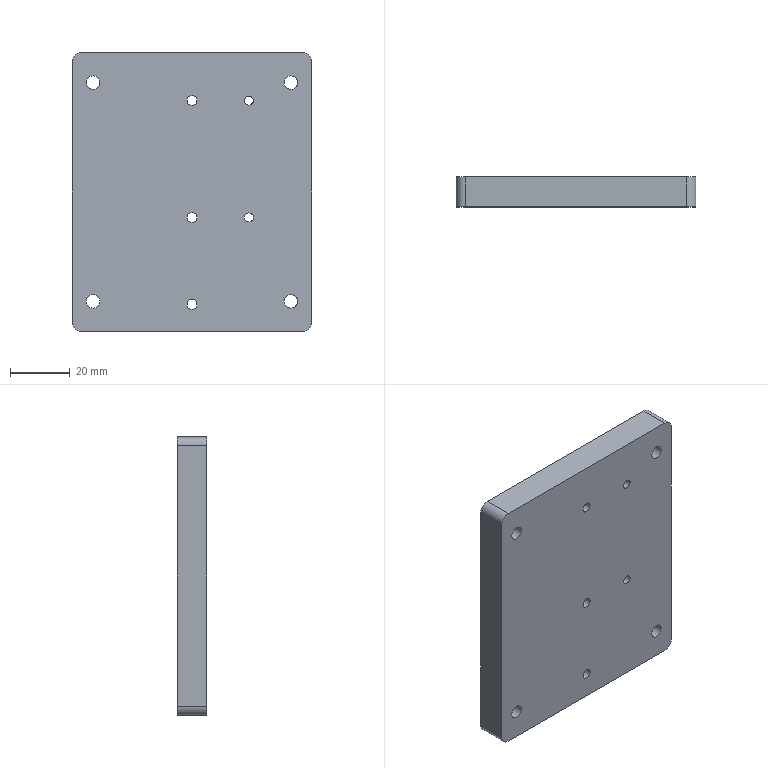Part | NX | 1 solid | 35 faces | box 80 x 10 x 93 mm | volume 72623 mm3 | cylinder 19 | plane 14 | cone 2 | commonest cylinder face diameters 4.5 x4 6 x4 8 x4 3.3 x3 3 x2 4 x2
STEP:
#1=CARTESIAN_POINT('',(104.923,-23.608,-66.529));
#2=VERTEX_POINT('',#1);
#3=CARTESIAN_POINT('',(101.923,-23.608,-69.529));
#4=VERTEX_POINT('',#3);
#5=CARTESIAN_POINT('',(104.923,-23.608,-69.529));
#6=DIRECTION('',(0.000000698,-1.,0.));
#7=DIRECTION('',(-0.000000349,0.,-1.));
#8=AXIS2_PLACEMENT_3D('',#5,#6,#7);
#9=CIRCLE('',#8,3.);
#10=EDGE_CURVE('',#2,#4,#9,.T.);
#11=ORIENTED_EDGE('',*,*,#10,.F.);
#12=CARTESIAN_POINT('',(104.923,-13.608,-66.529));
#13=VERTEX_POINT('',#12);
#14=CARTESIAN_POINT('',(104.923,-23.608,-66.529));
#15=DIRECTION('',(0.000000698,-1.,0.));
#16=VECTOR('',#15,1000.);
#17=LINE('',#14,#16);
#18=EDGE_CURVE('',#13,#2,#17,.T.);
#19=ORIENTED_EDGE('',*,*,#18,.F.);
#20=CARTESIAN_POINT('',(101.923,-13.608,-69.529));
#21=VERTEX_POINT('',#20);
#22=CARTESIAN_POINT('',(104.923,-13.608,-69.529));
#23=DIRECTION('',(-0.000000698,1.,0.));
#24=DIRECTION('',(-0.000000349,0.,-1.));
#25=AXIS2_PLACEMENT_3D('',#22,#23,#24);
#26=CIRCLE('',#25,3.);
#27=EDGE_CURVE('',#21,#13,#26,.T.);
#28=ORIENTED_EDGE('',*,*,#27,.F.);
#29=CARTESIAN_POINT('',(101.923,-24.294,-69.529));
#30=DIRECTION('',(-0.000000698,1.,0.));
#31=VECTOR('',#30,1000.);
#32=LINE('',#29,#31);
#33=EDGE_CURVE('',#4,#21,#32,.T.);
#34=ORIENTED_EDGE('',*,*,#33,.F.);
#35=EDGE_LOOP('',(#11,#19,#28,#34));
#36=FACE_BOUND('',#35,.T.);
#37=CARTESIAN_POINT('',(104.923,-23.608,-69.529));
#38=DIRECTION('',(0.000000698,-1.,0.));
#39=DIRECTION('',(-0.000000349,0.,-1.));
#40=AXIS2_PLACEMENT_3D('',#37,#38,#39);
#41=CYLINDRICAL_SURFACE('',#40,3.);
#42=ADVANCED_FACE('',(#36),#41,.T.);
#43=CARTESIAN_POINT('',(101.923,-23.608,-156.529));
#44=VERTEX_POINT('',#43);
#45=CARTESIAN_POINT('',(104.923,-23.608,-159.529));
#46=VERTEX_POINT('',#45);
#47=CARTESIAN_POINT('',(104.923,-23.608,-156.529));
#48=DIRECTION('',(0.000000698,-1.,0.));
#49=DIRECTION('',(-0.000000349,0.,-1.));
#50=AXIS2_PLACEMENT_3D('',#47,#48,#49);
#51=CIRCLE('',#50,3.);
#52=EDGE_CURVE('',#44,#46,#51,.T.);
#53=ORIENTED_EDGE('',*,*,#52,.F.);
#54=CARTESIAN_POINT('',(101.923,-13.608,-156.529));
#55=VERTEX_POINT('',#54);
#56=CARTESIAN_POINT('',(101.923,-24.294,-156.529));
#57=DIRECTION('',(0.000000698,-1.,0.));
#58=VECTOR('',#57,1000.);
#59=LINE('',#56,#58);
#60=EDGE_CURVE('',#55,#44,#59,.T.);
#61=ORIENTED_EDGE('',*,*,#60,.F.);
#62=CARTESIAN_POINT('',(104.923,-13.608,-159.529));
#63=VERTEX_POINT('',#62);
#64=CARTESIAN_POINT('',(104.923,-13.608,-156.529));
#65=DIRECTION('',(-0.000000698,1.,0.));
#66=DIRECTION('',(-0.000000349,0.,-1.));
#67=AXIS2_PLACEMENT_3D('',#64,#65,#66);
#68=CIRCLE('',#67,3.);
#69=EDGE_CURVE('',#63,#55,#68,.T.);
#70=ORIENTED_EDGE('',*,*,#69,.F.);
#71=CARTESIAN_POINT('',(104.923,-23.608,-159.529));
#72=DIRECTION('',(-0.000000698,1.,0.));
#73=VECTOR('',#72,1000.);
#74=LINE('',#71,#73);
#75=EDGE_CURVE('',#46,#63,#74,.T.);
#76=ORIENTED_EDGE('',*,*,#75,.F.);
#77=EDGE_LOOP('',(#53,#61,#70,#76));
#78=FACE_BOUND('',#77,.T.);
#79=CARTESIAN_POINT('',(104.923,-24.294,-156.529));
#80=DIRECTION('',(0.000000698,-1.,0.));
#81=DIRECTION('',(-0.000000349,0.,-1.));
#82=AXIS2_PLACEMENT_3D('',#79,#80,#81);
#83=CYLINDRICAL_SURFACE('',#82,3.);
#84=ADVANCED_FACE('',(#78),#83,.T.);
#85=CARTESIAN_POINT('',(178.923,-23.608,-159.529));
#86=VERTEX_POINT('',#85);
#87=CARTESIAN_POINT('',(181.923,-23.608,-156.529));
#88=VERTEX_POINT('',#87);
#89=CARTESIAN_POINT('',(178.923,-23.608,-156.529));
#90=DIRECTION('',(0.000000698,-1.,0.));
#91=DIRECTION('',(-0.000000349,0.,-1.));
#92=AXIS2_PLACEMENT_3D('',#89,#90,#91);
#93=CIRCLE('',#92,3.);
#94=EDGE_CURVE('',#86,#88,#93,.T.);
#95=ORIENTED_EDGE('',*,*,#94,.F.);
#96=CARTESIAN_POINT('',(178.923,-13.608,-159.529));
#97=VERTEX_POINT('',#96);
#98=CARTESIAN_POINT('',(178.923,-23.608,-159.529));
#99=DIRECTION('',(0.000000698,-1.,0.));
#100=VECTOR('',#99,1000.);
#101=LINE('',#98,#100);
#102=EDGE_CURVE('',#97,#86,#101,.T.);
#103=ORIENTED_EDGE('',*,*,#102,.F.);
#104=CARTESIAN_POINT('',(181.923,-13.608,-156.529));
#105=VERTEX_POINT('',#104);
#106=CARTESIAN_POINT('',(178.923,-13.608,-156.529));
#107=DIRECTION('',(-0.000000698,1.,0.));
#108=DIRECTION('',(-0.000000349,0.,-1.));
#109=AXIS2_PLACEMENT_3D('',#106,#107,#108);
#110=CIRCLE('',#109,3.);
#111=EDGE_CURVE('',#105,#97,#110,.T.);
#112=ORIENTED_EDGE('',*,*,#111,.F.);
#113=CARTESIAN_POINT('',(181.923,-24.294,-156.529));
#114=DIRECTION('',(-0.000000698,1.,0.));
#115=VECTOR('',#114,1000.);
#116=LINE('',#113,#115);
#117=EDGE_CURVE('',#88,#105,#116,.T.);
#118=ORIENTED_EDGE('',*,*,#117,.F.);
#119=EDGE_LOOP('',(#95,#103,#112,#118));
#120=FACE_BOUND('',#119,.T.);
#121=CARTESIAN_POINT('',(178.923,-23.608,-156.529));
#122=DIRECTION('',(-0.000000698,1.,0.));
#123=DIRECTION('',(0.000000349,0.,1.));
#124=AXIS2_PLACEMENT_3D('',#121,#122,#123);
#125=CYLINDRICAL_SURFACE('',#124,3.);
#126=ADVANCED_FACE('',(#120),#125,.T.);
#127=CARTESIAN_POINT('',(181.923,-23.608,-69.529));
#128=VERTEX_POINT('',#127);
#129=CARTESIAN_POINT('',(178.923,-23.608,-66.529));
#130=VERTEX_POINT('',#129);
#131=CARTESIAN_POINT('',(178.923,-23.608,-69.529));
#132=DIRECTION('',(0.000000698,-1.,0.));
#133=DIRECTION('',(-0.000000349,0.,-1.));
#134=AXIS2_PLACEMENT_3D('',#131,#132,#133);
#135=CIRCLE('',#134,3.);
#136=EDGE_CURVE('',#128,#130,#135,.T.);
#137=ORIENTED_EDGE('',*,*,#136,.F.);
#138=CARTESIAN_POINT('',(181.923,-13.608,-69.529));
#139=VERTEX_POINT('',#138);
#140=CARTESIAN_POINT('',(181.923,-24.294,-69.529));
#141=DIRECTION('',(0.000000698,-1.,0.));
#142=VECTOR('',#141,1000.);
#143=LINE('',#140,#142);
#144=EDGE_CURVE('',#139,#128,#143,.T.);
#145=ORIENTED_EDGE('',*,*,#144,.F.);
#146=CARTESIAN_POINT('',(178.923,-13.608,-66.529));
#147=VERTEX_POINT('',#146);
#148=CARTESIAN_POINT('',(178.923,-13.608,-69.529));
#149=DIRECTION('',(-0.000000698,1.,0.));
#150=DIRECTION('',(-0.000000349,0.,-1.));
#151=AXIS2_PLACEMENT_3D('',#148,#149,#150);
#152=CIRCLE('',#151,3.);
#153=EDGE_CURVE('',#147,#139,#152,.T.);
#154=ORIENTED_EDGE('',*,*,#153,.F.);
#155=CARTESIAN_POINT('',(178.923,-23.608,-66.529));
#156=DIRECTION('',(-0.000000698,1.,0.));
#157=VECTOR('',#156,1000.);
#158=LINE('',#155,#157);
#159=EDGE_CURVE('',#130,#147,#158,.T.);
#160=ORIENTED_EDGE('',*,*,#159,.F.);
#161=EDGE_LOOP('',(#137,#145,#154,#160));
#162=FACE_BOUND('',#161,.T.);
#163=CARTESIAN_POINT('',(178.923,-24.294,-69.529));
#164=DIRECTION('',(-0.000000698,1.,0.));
#165=DIRECTION('',(0.000000349,0.,1.));
#166=AXIS2_PLACEMENT_3D('',#163,#164,#165);
#167=CYLINDRICAL_SURFACE('',#166,3.);
#168=ADVANCED_FACE('',(#162),#167,.T.);
#169=CARTESIAN_POINT('',(162.923,-18.608,-82.529));
#170=VERTEX_POINT('',#169);
#171=CARTESIAN_POINT('',(160.923,-18.608,-82.529));
#172=DIRECTION('',(-0.000000698,1.,0.));
#173=DIRECTION('',(1.,0.000000698,0.));
#174=AXIS2_PLACEMENT_3D('',#171,#172,#173);
#175=CIRCLE('',#174,2.);
#176=EDGE_CURVE('',#170,#170,#175,.T.);
#177=ORIENTED_EDGE('',*,*,#176,.T.);
#178=EDGE_LOOP('',(#177));
#179=FACE_BOUND('',#178,.T.);
#180=CARTESIAN_POINT('',(162.423,-18.608,-82.529));
#181=VERTEX_POINT('',#180);
#182=CARTESIAN_POINT('',(160.923,-18.608,-82.529));
#183=DIRECTION('',(-0.000000698,1.,0.));
#184=DIRECTION('',(1.,0.000000698,0.));
#185=AXIS2_PLACEMENT_3D('',#182,#183,#184);
#186=CIRCLE('',#185,1.5);
#187=EDGE_CURVE('',#181,#181,#186,.T.);
#188=ORIENTED_EDGE('',*,*,#187,.F.);
#189=EDGE_LOOP('',(#188));
#190=FACE_BOUND('',#189,.T.);
#191=CARTESIAN_POINT('',(160.923,-18.608,-123.029));
#192=DIRECTION('',(0.000000698,-1.,0.));
#193=DIRECTION('',(0.,0.,-1.));
#194=AXIS2_PLACEMENT_3D('',#191,#192,#193);
#195=PLANE('',#194);
#196=ADVANCED_FACE('',(#179,#190),#195,.F.);
#197=CARTESIAN_POINT('',(160.923,-18.608,-119.529));
#198=VERTEX_POINT('',#197);
#199=CARTESIAN_POINT('',(160.923,-18.608,-121.529));
#200=DIRECTION('',(-0.000000698,1.,0.));
#201=DIRECTION('',(0.,0.,1.));
#202=AXIS2_PLACEMENT_3D('',#199,#200,#201);
#203=CIRCLE('',#202,2.);
#204=EDGE_CURVE('',#198,#198,#203,.T.);
#205=ORIENTED_EDGE('',*,*,#204,.T.);
#206=EDGE_LOOP('',(#205));
#207=FACE_BOUND('',#206,.T.);
#208=CARTESIAN_POINT('',(160.923,-18.608,-120.029));
#209=VERTEX_POINT('',#208);
#210=CARTESIAN_POINT('',(160.923,-18.608,-121.529));
#211=DIRECTION('',(-0.000000698,1.,0.));
#212=DIRECTION('',(0.,0.,1.));
#213=AXIS2_PLACEMENT_3D('',#210,#211,#212);
#214=CIRCLE('',#213,1.5);
#215=EDGE_CURVE('',#209,#209,#214,.T.);
#216=ORIENTED_EDGE('',*,*,#215,.F.);
#217=EDGE_LOOP('',(#216));
#218=FACE_BOUND('',#217,.T.);
#219=CARTESIAN_POINT('',(160.923,-18.608,-123.029));
#220=DIRECTION('',(0.000000698,-1.,0.));
#221=DIRECTION('',(0.,0.,-1.));
#222=AXIS2_PLACEMENT_3D('',#219,#220,#221);
#223=PLANE('',#222);
#224=ADVANCED_FACE('',(#207,#218),#223,.F.);
#225=CARTESIAN_POINT('',(178.923,-18.008,-149.529));
#226=VERTEX_POINT('',#225);
#227=CARTESIAN_POINT('',(174.923,-18.008,-149.529));
#228=DIRECTION('',(-0.000000698,1.,0.));
#229=DIRECTION('',(1.,0.000000698,0.));
#230=AXIS2_PLACEMENT_3D('',#227,#228,#229);
#231=CIRCLE('',#230,4.);
#232=EDGE_CURVE('',#226,#226,#231,.T.);
#233=ORIENTED_EDGE('',*,*,#232,.T.);
#234=EDGE_LOOP('',(#233));
#235=FACE_BOUND('',#234,.T.);
#236=CARTESIAN_POINT('',(177.173,-18.008,-149.529));
#237=VERTEX_POINT('',#236);
#238=CARTESIAN_POINT('',(174.923,-18.008,-149.529));
#239=DIRECTION('',(-0.000000698,1.,0.));
#240=DIRECTION('',(1.,0.000000698,0.));
#241=AXIS2_PLACEMENT_3D('',#238,#239,#240);
#242=CIRCLE('',#241,2.25);
#243=EDGE_CURVE('',#237,#237,#242,.T.);
#244=ORIENTED_EDGE('',*,*,#243,.F.);
#245=EDGE_LOOP('',(#244));
#246=FACE_BOUND('',#245,.T.);
#247=CARTESIAN_POINT('',(108.923,-18.008,-151.779));
#248=DIRECTION('',(0.000000698,-1.,0.));
#249=DIRECTION('',(0.,0.,-1.));
#250=AXIS2_PLACEMENT_3D('',#247,#248,#249);
#251=PLANE('',#250);
#252=ADVANCED_FACE('',(#235,#246),#251,.F.);
#253=CARTESIAN_POINT('',(178.923,-18.008,-76.529));
#254=VERTEX_POINT('',#253);
#255=CARTESIAN_POINT('',(174.923,-18.008,-76.529));
#256=DIRECTION('',(-0.000000698,1.,0.));
#257=DIRECTION('',(1.,0.000000698,0.));
#258=AXIS2_PLACEMENT_3D('',#255,#256,#257);
#259=CIRCLE('',#258,4.);
#260=EDGE_CURVE('',#254,#254,#259,.T.);
#261=ORIENTED_EDGE('',*,*,#260,.T.);
#262=EDGE_LOOP('',(#261));
#263=FACE_BOUND('',#262,.T.);
#264=CARTESIAN_POINT('',(177.173,-18.008,-76.529));
#265=VERTEX_POINT('',#264);
#266=CARTESIAN_POINT('',(174.923,-18.008,-76.529));
#267=DIRECTION('',(-0.000000698,1.,0.));
#268=DIRECTION('',(1.,0.000000698,0.));
#269=AXIS2_PLACEMENT_3D('',#266,#267,#268);
#270=CIRCLE('',#269,2.25);
#271=EDGE_CURVE('',#265,#265,#270,.T.);
#272=ORIENTED_EDGE('',*,*,#271,.F.);
#273=EDGE_LOOP('',(#272));
#274=FACE_BOUND('',#273,.T.);
#275=CARTESIAN_POINT('',(108.923,-18.008,-151.779));
#276=DIRECTION('',(0.000000698,-1.,0.));
#277=DIRECTION('',(0.,0.,-1.));
#278=AXIS2_PLACEMENT_3D('',#275,#276,#277);
#279=PLANE('',#278);
#280=ADVANCED_FACE('',(#263,#274),#279,.F.);
#281=CARTESIAN_POINT('',(112.923,-18.008,-76.529));
#282=VERTEX_POINT('',#281);
#283=CARTESIAN_POINT('',(108.923,-18.008,-76.529));
#284=DIRECTION('',(-0.000000698,1.,0.));
#285=DIRECTION('',(1.,0.000000698,0.));
#286=AXIS2_PLACEMENT_3D('',#283,#284,#285);
#287=CIRCLE('',#286,4.);
#288=EDGE_CURVE('',#282,#282,#287,.T.);
#289=ORIENTED_EDGE('',*,*,#288,.T.);
#290=EDGE_LOOP('',(#289));
#291=FACE_BOUND('',#290,.T.);
#292=CARTESIAN_POINT('',(111.173,-18.008,-76.529));
#293=VERTEX_POINT('',#292);
#294=CARTESIAN_POINT('',(108.923,-18.008,-76.529));
#295=DIRECTION('',(-0.000000698,1.,0.));
#296=DIRECTION('',(1.,0.000000698,0.));
#297=AXIS2_PLACEMENT_3D('',#294,#295,#296);
#298=CIRCLE('',#297,2.25);
#299=EDGE_CURVE('',#293,#293,#298,.T.);
#300=ORIENTED_EDGE('',*,*,#299,.F.);
#301=EDGE_LOOP('',(#300));
#302=FACE_BOUND('',#301,.T.);
#303=CARTESIAN_POINT('',(108.923,-18.008,-151.779));
#304=DIRECTION('',(0.000000698,-1.,0.));
#305=DIRECTION('',(0.,0.,-1.));
#306=AXIS2_PLACEMENT_3D('',#303,#304,#305);
#307=PLANE('',#306);
#308=ADVANCED_FACE('',(#291,#302),#307,.F.);
#309=CARTESIAN_POINT('',(108.923,-18.008,-145.529));
#310=VERTEX_POINT('',#309);
#311=CARTESIAN_POINT('',(108.923,-18.008,-149.529));
#312=DIRECTION('',(-0.000000698,1.,0.));
#313=DIRECTION('',(0.,0.,1.));
#314=AXIS2_PLACEMENT_3D('',#311,#312,#313);
#315=CIRCLE('',#314,4.);
#316=EDGE_CURVE('',#310,#310,#315,.T.);
#317=ORIENTED_EDGE('',*,*,#316,.T.);
#318=EDGE_LOOP('',(#317));
#319=FACE_BOUND('',#318,.T.);
#320=CARTESIAN_POINT('',(108.923,-18.008,-147.279));
#321=VERTEX_POINT('',#320);
#322=CARTESIAN_POINT('',(108.923,-18.008,-149.529));
#323=DIRECTION('',(-0.000000698,1.,0.));
#324=DIRECTION('',(0.,0.,1.));
#325=AXIS2_PLACEMENT_3D('',#322,#323,#324);
#326=CIRCLE('',#325,2.25);
#327=EDGE_CURVE('',#321,#321,#326,.T.);
#328=ORIENTED_EDGE('',*,*,#327,.F.);
#329=EDGE_LOOP('',(#328));
#330=FACE_BOUND('',#329,.T.);
#331=CARTESIAN_POINT('',(108.923,-18.008,-151.779));
#332=DIRECTION('',(0.000000698,-1.,0.));
#333=DIRECTION('',(0.,0.,-1.));
#334=AXIS2_PLACEMENT_3D('',#331,#332,#333);
#335=PLANE('',#334);
#336=ADVANCED_FACE('',(#319,#330),#335,.F.);
#337=CARTESIAN_POINT('',(105.923,-13.608,-66.529));
#338=DIRECTION('',(-1.,-0.000000698,0.));
#339=VECTOR('',#338,1000.);
#340=LINE('',#337,#339);
#341=EDGE_CURVE('',#147,#13,#340,.T.);
#342=ORIENTED_EDGE('',*,*,#341,.F.);
#343=ORIENTED_EDGE('',*,*,#153,.T.);
#344=CARTESIAN_POINT('',(181.923,-13.608,-112.251));
#345=DIRECTION('',(0.,0.,1.));
#346=VECTOR('',#345,1000.);
#347=LINE('',#344,#346);
#348=EDGE_CURVE('',#105,#139,#347,.T.);
#349=ORIENTED_EDGE('',*,*,#348,.F.);
#350=ORIENTED_EDGE('',*,*,#111,.T.);
#351=CARTESIAN_POINT('',(105.923,-13.608,-159.529));
#352=DIRECTION('',(1.,0.000000698,0.));
#353=VECTOR('',#352,1000.);
#354=LINE('',#351,#353);
#355=EDGE_CURVE('',#63,#97,#354,.T.);
#356=ORIENTED_EDGE('',*,*,#355,.F.);
#357=ORIENTED_EDGE('',*,*,#69,.T.);
#358=CARTESIAN_POINT('',(101.923,-13.608,-112.251));
#359=DIRECTION('',(0.,0.,-1.));
#360=VECTOR('',#359,1000.);
#361=LINE('',#358,#360);
#362=EDGE_CURVE('',#21,#55,#361,.T.);
#363=ORIENTED_EDGE('',*,*,#362,.F.);
#364=ORIENTED_EDGE('',*,*,#27,.T.);
#365=EDGE_LOOP('',(#342,#343,#349,#350,#356,#357,#363,#364));
#366=FACE_BOUND('',#365,.T.);
#367=CARTESIAN_POINT('',(141.923,-13.608,-80.879));
#368=VERTEX_POINT('',#367);
#369=CARTESIAN_POINT('',(141.923,-13.608,-82.529));
#370=DIRECTION('',(-0.000000698,1.,0.));
#371=DIRECTION('',(0.,0.,1.));
#372=AXIS2_PLACEMENT_3D('',#369,#370,#371);
#373=CIRCLE('',#372,1.65);
#374=EDGE_CURVE('',#368,#368,#373,.T.);
#375=ORIENTED_EDGE('',*,*,#374,.F.);
#376=EDGE_LOOP('',(#375));
#377=FACE_BOUND('',#376,.T.);
#378=CARTESIAN_POINT('',(141.923,-13.608,-148.879));
#379=VERTEX_POINT('',#378);
#380=CARTESIAN_POINT('',(141.923,-13.608,-150.529));
#381=DIRECTION('',(-0.000000698,1.,0.));
#382=DIRECTION('',(0.,0.,1.));
#383=AXIS2_PLACEMENT_3D('',#380,#381,#382);
#384=CIRCLE('',#383,1.65);
#385=EDGE_CURVE('',#379,#379,#384,.T.);
#386=ORIENTED_EDGE('',*,*,#385,.F.);
#387=EDGE_LOOP('',(#386));
#388=FACE_BOUND('',#387,.T.);
#389=CARTESIAN_POINT('',(141.923,-13.608,-119.879));
#390=VERTEX_POINT('',#389);
#391=CARTESIAN_POINT('',(141.923,-13.608,-121.529));
#392=DIRECTION('',(-0.000000698,1.,0.));
#393=DIRECTION('',(0.,0.,1.));
#394=AXIS2_PLACEMENT_3D('',#391,#392,#393);
#395=CIRCLE('',#394,1.65);
#396=EDGE_CURVE('',#390,#390,#395,.T.);
#397=ORIENTED_EDGE('',*,*,#396,.F.);
#398=EDGE_LOOP('',(#397));
#399=FACE_BOUND('',#398,.T.);
#400=CARTESIAN_POINT('',(108.923,-13.608,-145.529));
#401=VERTEX_POINT('',#400);
#402=CARTESIAN_POINT('',(108.923,-13.608,-149.529));
#403=DIRECTION('',(-0.000000698,1.,0.));
#404=DIRECTION('',(0.,0.,1.));
#405=AXIS2_PLACEMENT_3D('',#402,#403,#404);
#406=CIRCLE('',#405,4.);
#407=EDGE_CURVE('',#401,#401,#406,.T.);
#408=ORIENTED_EDGE('',*,*,#407,.F.);
#409=EDGE_LOOP('',(#408));
#410=FACE_BOUND('',#409,.T.);
#411=CARTESIAN_POINT('',(108.923,-13.608,-72.529));
#412=VERTEX_POINT('',#411);
#413=CARTESIAN_POINT('',(108.923,-13.608,-76.529));
#414=DIRECTION('',(-0.000000698,1.,0.));
#415=DIRECTION('',(0.,0.,1.));
#416=AXIS2_PLACEMENT_3D('',#413,#414,#415);
#417=CIRCLE('',#416,4.);
#418=EDGE_CURVE('',#412,#412,#417,.T.);
#419=ORIENTED_EDGE('',*,*,#418,.F.);
#420=EDGE_LOOP('',(#419));
#421=FACE_BOUND('',#420,.T.);
#422=CARTESIAN_POINT('',(174.923,-13.608,-72.529));
#423=VERTEX_POINT('',#422);
#424=CARTESIAN_POINT('',(174.923,-13.608,-76.529));
#425=DIRECTION('',(-0.000000698,1.,0.));
#426=DIRECTION('',(0.,0.,1.));
#427=AXIS2_PLACEMENT_3D('',#424,#425,#426);
#428=CIRCLE('',#427,4.);
#429=EDGE_CURVE('',#423,#423,#428,.T.);
#430=ORIENTED_EDGE('',*,*,#429,.F.);
#431=EDGE_LOOP('',(#430));
#432=FACE_BOUND('',#431,.T.);
#433=CARTESIAN_POINT('',(174.923,-13.608,-145.529));
#434=VERTEX_POINT('',#433);
#435=CARTESIAN_POINT('',(174.923,-13.608,-149.529));
#436=DIRECTION('',(-0.000000698,1.,0.));
#437=DIRECTION('',(0.,0.,1.));
#438=AXIS2_PLACEMENT_3D('',#435,#436,#437);
#439=CIRCLE('',#438,4.);
#440=EDGE_CURVE('',#434,#434,#439,.T.);
#441=ORIENTED_EDGE('',*,*,#440,.F.);
#442=EDGE_LOOP('',(#441));
#443=FACE_BOUND('',#442,.T.);
#444=CARTESIAN_POINT('',(160.923,-13.608,-119.529));
#445=VERTEX_POINT('',#444);
#446=CARTESIAN_POINT('',(160.923,-13.608,-121.529));
#447=DIRECTION('',(-0.000000698,1.,0.));
#448=DIRECTION('',(0.,0.,1.));
#449=AXIS2_PLACEMENT_3D('',#446,#447,#448);
#450=CIRCLE('',#449,2.);
#451=EDGE_CURVE('',#445,#445,#450,.T.);
#452=ORIENTED_EDGE('',*,*,#451,.F.);
#453=EDGE_LOOP('',(#452));
#454=FACE_BOUND('',#453,.T.);
#455=CARTESIAN_POINT('',(160.923,-13.608,-80.529));
#456=VERTEX_POINT('',#455);
#457=CARTESIAN_POINT('',(160.923,-13.608,-82.529));
#458=DIRECTION('',(-0.000000698,1.,0.));
#459=DIRECTION('',(0.,0.,1.));
#460=AXIS2_PLACEMENT_3D('',#457,#458,#459);
#461=CIRCLE('',#460,2.);
#462=EDGE_CURVE('',#456,#456,#461,.T.);
#463=ORIENTED_EDGE('',*,*,#462,.F.);
#464=EDGE_LOOP('',(#463));
#465=FACE_BOUND('',#464,.T.);
#466=CARTESIAN_POINT('',(141.923,-13.608,-113.029));
#467=DIRECTION('',(0.000000698,-1.,0.));
#468=DIRECTION('',(0.,0.,-1.));
#469=AXIS2_PLACEMENT_3D('',#466,#467,#468);
#470=PLANE('',#469);
#471=ADVANCED_FACE('',(#366,#377,#388,#399,#410,#421,#432,#443,#454,#465),#470,.F.);
#472=CARTESIAN_POINT('',(181.923,-23.608,-112.251));
#473=DIRECTION('',(0.,0.,1.));
#474=VECTOR('',#473,1000.);
#475=LINE('',#472,#474);
#476=EDGE_CURVE('',#88,#128,#475,.T.);
#477=ORIENTED_EDGE('',*,*,#476,.T.);
#478=ORIENTED_EDGE('',*,*,#136,.T.);
#479=CARTESIAN_POINT('',(105.923,-23.608,-66.529));
#480=DIRECTION('',(-1.,-0.000000698,0.));
#481=VECTOR('',#480,1000.);
#482=LINE('',#479,#481);
#483=EDGE_CURVE('',#130,#2,#482,.T.);
#484=ORIENTED_EDGE('',*,*,#483,.T.);
#485=ORIENTED_EDGE('',*,*,#10,.T.);
#486=CARTESIAN_POINT('',(101.923,-23.608,-112.251));
#487=DIRECTION('',(0.,0.,-1.));
#488=VECTOR('',#487,1000.);
#489=LINE('',#486,#488);
#490=EDGE_CURVE('',#4,#44,#489,.T.);
#491=ORIENTED_EDGE('',*,*,#490,.T.);
#492=ORIENTED_EDGE('',*,*,#52,.T.);
#493=CARTESIAN_POINT('',(105.923,-23.608,-159.529));
#494=DIRECTION('',(1.,0.000000698,0.));
#495=VECTOR('',#494,1000.);
#496=LINE('',#493,#495);
#497=EDGE_CURVE('',#46,#86,#496,.T.);
#498=ORIENTED_EDGE('',*,*,#497,.T.);
#499=ORIENTED_EDGE('',*,*,#94,.T.);
#500=EDGE_LOOP('',(#477,#478,#484,#485,#491,#492,#498,#499));
#501=FACE_BOUND('',#500,.T.);
#502=CARTESIAN_POINT('',(141.923,-23.608,-80.879));
#503=VERTEX_POINT('',#502);
#504=CARTESIAN_POINT('',(141.923,-23.608,-82.529));
#505=DIRECTION('',(-0.000000698,1.,0.));
#506=DIRECTION('',(0.,0.,1.));
#507=AXIS2_PLACEMENT_3D('',#504,#505,#506);
#508=CIRCLE('',#507,1.65);
#509=EDGE_CURVE('',#503,#503,#508,.T.);
#510=ORIENTED_EDGE('',*,*,#509,.T.);
#511=EDGE_LOOP('',(#510));
#512=FACE_BOUND('',#511,.T.);
#513=CARTESIAN_POINT('',(141.923,-23.608,-148.879));
#514=VERTEX_POINT('',#513);
#515=CARTESIAN_POINT('',(141.923,-23.608,-150.529));
#516=DIRECTION('',(-0.000000698,1.,0.));
#517=DIRECTION('',(0.,0.,1.));
#518=AXIS2_PLACEMENT_3D('',#515,#516,#517);
#519=CIRCLE('',#518,1.65);
#520=EDGE_CURVE('',#514,#514,#519,.T.);
#521=ORIENTED_EDGE('',*,*,#520,.T.);
#522=EDGE_LOOP('',(#521));
#523=FACE_BOUND('',#522,.T.);
#524=CARTESIAN_POINT('',(141.923,-23.608,-119.879));
#525=VERTEX_POINT('',#524);
#526=CARTESIAN_POINT('',(141.923,-23.608,-121.529));
#527=DIRECTION('',(-0.000000698,1.,0.));
#528=DIRECTION('',(0.,0.,1.));
#529=AXIS2_PLACEMENT_3D('',#526,#527,#528);
#530=CIRCLE('',#529,1.65);
#531=EDGE_CURVE('',#525,#525,#530,.T.);
#532=ORIENTED_EDGE('',*,*,#531,.T.);
#533=EDGE_LOOP('',(#532));
#534=FACE_BOUND('',#533,.T.);
#535=CARTESIAN_POINT('',(108.923,-23.608,-147.279));
#536=VERTEX_POINT('',#535);
#537=CARTESIAN_POINT('',(108.923,-23.608,-149.529));
#538=DIRECTION('',(-0.000000698,1.,0.));
#539=DIRECTION('',(0.,0.,1.));
#540=AXIS2_PLACEMENT_3D('',#537,#538,#539);
#541=CIRCLE('',#540,2.25);
#542=EDGE_CURVE('',#536,#536,#541,.T.);
#543=ORIENTED_EDGE('',*,*,#542,.T.);
#544=EDGE_LOOP('',(#543));
#545=FACE_BOUND('',#544,.T.);
#546=CARTESIAN_POINT('',(108.923,-23.608,-74.279));
#547=VERTEX_POINT('',#546);
#548=CARTESIAN_POINT('',(108.923,-23.608,-76.529));
#549=DIRECTION('',(-0.000000698,1.,0.));
#550=DIRECTION('',(0.,0.,1.));
#551=AXIS2_PLACEMENT_3D('',#548,#549,#550);
#552=CIRCLE('',#551,2.25);
#553=EDGE_CURVE('',#547,#547,#552,.T.);
#554=ORIENTED_EDGE('',*,*,#553,.T.);
#555=EDGE_LOOP('',(#554));
#556=FACE_BOUND('',#555,.T.);
#557=CARTESIAN_POINT('',(174.923,-23.608,-74.279));
#558=VERTEX_POINT('',#557);
#559=CARTESIAN_POINT('',(174.923,-23.608,-76.529));
#560=DIRECTION('',(-0.000000698,1.,0.));
#561=DIRECTION('',(0.,0.,1.));
#562=AXIS2_PLACEMENT_3D('',#559,#560,#561);
#563=CIRCLE('',#562,2.25);
#564=EDGE_CURVE('',#558,#558,#563,.T.);
#565=ORIENTED_EDGE('',*,*,#564,.T.);
#566=EDGE_LOOP('',(#565));
#567=FACE_BOUND('',#566,.T.);
#568=CARTESIAN_POINT('',(174.923,-23.608,-147.279));
#569=VERTEX_POINT('',#568);
#570=CARTESIAN_POINT('',(174.923,-23.608,-149.529));
#571=DIRECTION('',(-0.000000698,1.,0.));
#572=DIRECTION('',(0.,0.,1.));
#573=AXIS2_PLACEMENT_3D('',#570,#571,#572);
#574=CIRCLE('',#573,2.25);
#575=EDGE_CURVE('',#569,#569,#574,.T.);
#576=ORIENTED_EDGE('',*,*,#575,.T.);
#577=EDGE_LOOP('',(#576));
#578=FACE_BOUND('',#577,.T.);
#579=CARTESIAN_POINT('',(160.923,-23.608,-120.029));
#580=VERTEX_POINT('',#579);
#581=CARTESIAN_POINT('',(160.923,-23.608,-121.529));
#582=DIRECTION('',(-0.000000698,1.,0.));
#583=DIRECTION('',(0.,0.,1.));
#584=AXIS2_PLACEMENT_3D('',#581,#582,#583);
#585=CIRCLE('',#584,1.5);
#586=EDGE_CURVE('',#580,#580,#585,.T.);
#587=ORIENTED_EDGE('',*,*,#586,.T.);
#588=EDGE_LOOP('',(#587));
#589=FACE_BOUND('',#588,.T.);
#590=CARTESIAN_POINT('',(160.923,-23.608,-81.029));
#591=VERTEX_POINT('',#590);
#592=CARTESIAN_POINT('',(160.923,-23.608,-82.529));
#593=DIRECTION('',(-0.000000698,1.,0.));
#594=DIRECTION('',(0.,0.,1.));
#595=AXIS2_PLACEMENT_3D('',#592,#593,#594);
#596=CIRCLE('',#595,1.5);
#597=EDGE_CURVE('',#591,#591,#596,.T.);
#598=ORIENTED_EDGE('',*,*,#597,.T.);
#599=EDGE_LOOP('',(#598));
#600=FACE_BOUND('',#599,.T.);
#601=CARTESIAN_POINT('',(141.923,-23.608,-113.029));
#602=DIRECTION('',(0.000000698,-1.,0.));
#603=DIRECTION('',(0.,0.,-1.));
#604=AXIS2_PLACEMENT_3D('',#601,#602,#603);
#605=PLANE('',#604);
#606=ADVANCED_FACE('',(#501,#512,#523,#534,#545,#556,#567,#578,#589,#600),#605,.T.);
#607=ORIENTED_EDGE('',*,*,#348,.T.);
#608=ORIENTED_EDGE('',*,*,#144,.T.);
#609=ORIENTED_EDGE('',*,*,#476,.F.);
#610=ORIENTED_EDGE('',*,*,#117,.T.);
#611=EDGE_LOOP('',(#607,#608,#609,#610));
#612=FACE_BOUND('',#611,.T.);
#613=CARTESIAN_POINT('',(181.923,-24.294,-112.251));
#614=DIRECTION('',(1.,0.000000698,0.));
#615=DIRECTION('',(0.,0.,-1.));
#616=AXIS2_PLACEMENT_3D('',#613,#614,#615);
#617=PLANE('',#616);
#618=ADVANCED_FACE('',(#612),#617,.T.);
#619=ORIENTED_EDGE('',*,*,#355,.T.);
#620=ORIENTED_EDGE('',*,*,#102,.T.);
#621=ORIENTED_EDGE('',*,*,#497,.F.);
#622=ORIENTED_EDGE('',*,*,#75,.T.);
#623=EDGE_LOOP('',(#619,#620,#621,#622));
#624=FACE_BOUND('',#623,.T.);
#625=CARTESIAN_POINT('',(105.923,-23.608,-159.529));
#626=DIRECTION('',(0.,0.,1.));
#627=DIRECTION('',(1.,0.,0.));
#628=AXIS2_PLACEMENT_3D('',#625,#626,#627);
#629=PLANE('',#628);
#630=ADVANCED_FACE('',(#624),#629,.F.);
#631=ORIENTED_EDGE('',*,*,#362,.T.);
#632=ORIENTED_EDGE('',*,*,#60,.T.);
#633=ORIENTED_EDGE('',*,*,#490,.F.);
#634=ORIENTED_EDGE('',*,*,#33,.T.);
#635=EDGE_LOOP('',(#631,#632,#633,#634));
#636=FACE_BOUND('',#635,.T.);
#637=CARTESIAN_POINT('',(101.923,-24.294,-112.251));
#638=DIRECTION('',(1.,0.000000698,0.));
#639=DIRECTION('',(0.,0.,-1.));
#640=AXIS2_PLACEMENT_3D('',#637,#638,#639);
#641=PLANE('',#640);
#642=ADVANCED_FACE('',(#636),#641,.F.);
#643=ORIENTED_EDGE('',*,*,#483,.F.);
#644=ORIENTED_EDGE('',*,*,#159,.T.);
#645=ORIENTED_EDGE('',*,*,#341,.T.);
#646=ORIENTED_EDGE('',*,*,#18,.T.);
#647=EDGE_LOOP('',(#643,#644,#645,#646));
#648=FACE_BOUND('',#647,.T.);
#649=CARTESIAN_POINT('',(105.923,-23.608,-66.529));
#650=DIRECTION('',(0.,0.,-1.));
#651=DIRECTION('',(0.,-1.,0.));
#652=AXIS2_PLACEMENT_3D('',#649,#650,#651);
#653=PLANE('',#652);
#654=ADVANCED_FACE('',(#648),#653,.F.);
#655=ORIENTED_EDGE('',*,*,#509,.F.);
#656=EDGE_LOOP('',(#655));
#657=FACE_BOUND('',#656,.T.);
#658=ORIENTED_EDGE('',*,*,#374,.T.);
#659=EDGE_LOOP('',(#658));
#660=FACE_BOUND('',#659,.T.);
#661=CARTESIAN_POINT('',(141.923,-13.608,-82.529));
#662=DIRECTION('',(-0.000000698,1.,0.));
#663=DIRECTION('',(0.,0.,1.));
#664=AXIS2_PLACEMENT_3D('',#661,#662,#663);
#665=CYLINDRICAL_SURFACE('',#664,1.65);
#666=ADVANCED_FACE('',(#657,#660),#665,.F.);
#667=ORIENTED_EDGE('',*,*,#520,.F.);
#668=EDGE_LOOP('',(#667));
#669=FACE_BOUND('',#668,.T.);
#670=ORIENTED_EDGE('',*,*,#385,.T.);
#671=EDGE_LOOP('',(#670));
#672=FACE_BOUND('',#671,.T.);
#673=CARTESIAN_POINT('',(141.923,-13.608,-150.529));
#674=DIRECTION('',(-0.000000698,1.,0.));
#675=DIRECTION('',(0.,0.,1.));
#676=AXIS2_PLACEMENT_3D('',#673,#674,#675);
#677=CYLINDRICAL_SURFACE('',#676,1.65);
#678=ADVANCED_FACE('',(#669,#672),#677,.F.);
#679=ORIENTED_EDGE('',*,*,#531,.F.);
#680=EDGE_LOOP('',(#679));
#681=FACE_BOUND('',#680,.T.);
#682=ORIENTED_EDGE('',*,*,#396,.T.);
#683=EDGE_LOOP('',(#682));
#684=FACE_BOUND('',#683,.T.);
#685=CARTESIAN_POINT('',(141.923,-13.608,-121.529));
#686=DIRECTION('',(-0.000000698,1.,0.));
#687=DIRECTION('',(0.,0.,1.));
#688=AXIS2_PLACEMENT_3D('',#685,#686,#687);
#689=CYLINDRICAL_SURFACE('',#688,1.65);
#690=ADVANCED_FACE('',(#681,#684),#689,.F.);
#691=ORIENTED_EDGE('',*,*,#542,.F.);
#692=EDGE_LOOP('',(#691));
#693=FACE_BOUND('',#692,.T.);
#694=ORIENTED_EDGE('',*,*,#327,.T.);
#695=EDGE_LOOP('',(#694));
#696=FACE_BOUND('',#695,.T.);
#697=CARTESIAN_POINT('',(108.923,-13.608,-149.529));
#698=DIRECTION('',(-0.000000698,1.,0.));
#699=DIRECTION('',(0.,0.,1.));
#700=AXIS2_PLACEMENT_3D('',#697,#698,#699);
#701=CYLINDRICAL_SURFACE('',#700,2.25);
#702=ADVANCED_FACE('',(#693,#696),#701,.F.);
#703=ORIENTED_EDGE('',*,*,#316,.F.);
#704=EDGE_LOOP('',(#703));
#705=FACE_BOUND('',#704,.T.);
#706=ORIENTED_EDGE('',*,*,#407,.T.);
#707=EDGE_LOOP('',(#706));
#708=FACE_BOUND('',#707,.T.);
#709=CARTESIAN_POINT('',(108.923,-13.608,-149.529));
#710=DIRECTION('',(-0.000000698,1.,0.));
#711=DIRECTION('',(0.,0.,1.));
#712=AXIS2_PLACEMENT_3D('',#709,#710,#711);
#713=CYLINDRICAL_SURFACE('',#712,4.);
#714=ADVANCED_FACE('',(#705,#708),#713,.F.);
#715=ORIENTED_EDGE('',*,*,#553,.F.);
#716=EDGE_LOOP('',(#715));
#717=FACE_BOUND('',#716,.T.);
#718=ORIENTED_EDGE('',*,*,#299,.T.);
#719=EDGE_LOOP('',(#718));
#720=FACE_BOUND('',#719,.T.);
#721=CARTESIAN_POINT('',(108.923,-13.608,-76.529));
#722=DIRECTION('',(-0.000000698,1.,0.));
#723=DIRECTION('',(0.,0.,1.));
#724=AXIS2_PLACEMENT_3D('',#721,#722,#723);
#725=CYLINDRICAL_SURFACE('',#724,2.25);
#726=ADVANCED_FACE('',(#717,#720),#725,.F.);
#727=ORIENTED_EDGE('',*,*,#288,.F.);
#728=EDGE_LOOP('',(#727));
#729=FACE_BOUND('',#728,.T.);
#730=ORIENTED_EDGE('',*,*,#418,.T.);
#731=EDGE_LOOP('',(#730));
#732=FACE_BOUND('',#731,.T.);
#733=CARTESIAN_POINT('',(108.923,-13.608,-76.529));
#734=DIRECTION('',(-0.000000698,1.,0.));
#735=DIRECTION('',(0.,0.,1.));
#736=AXIS2_PLACEMENT_3D('',#733,#734,#735);
#737=CYLINDRICAL_SURFACE('',#736,4.);
#738=ADVANCED_FACE('',(#729,#732),#737,.F.);
#739=ORIENTED_EDGE('',*,*,#564,.F.);
#740=EDGE_LOOP('',(#739));
#741=FACE_BOUND('',#740,.T.);
#742=ORIENTED_EDGE('',*,*,#271,.T.);
#743=EDGE_LOOP('',(#742));
#744=FACE_BOUND('',#743,.T.);
#745=CARTESIAN_POINT('',(174.923,-13.608,-76.529));
#746=DIRECTION('',(-0.000000698,1.,0.));
#747=DIRECTION('',(0.,0.,1.));
#748=AXIS2_PLACEMENT_3D('',#745,#746,#747);
#749=CYLINDRICAL_SURFACE('',#748,2.25);
#750=ADVANCED_FACE('',(#741,#744),#749,.F.);
#751=ORIENTED_EDGE('',*,*,#260,.F.);
#752=EDGE_LOOP('',(#751));
#753=FACE_BOUND('',#752,.T.);
#754=ORIENTED_EDGE('',*,*,#429,.T.);
#755=EDGE_LOOP('',(#754));
#756=FACE_BOUND('',#755,.T.);
#757=CARTESIAN_POINT('',(174.923,-13.608,-76.529));
#758=DIRECTION('',(-0.000000698,1.,0.));
#759=DIRECTION('',(0.,0.,1.));
#760=AXIS2_PLACEMENT_3D('',#757,#758,#759);
#761=CYLINDRICAL_SURFACE('',#760,4.);
#762=ADVANCED_FACE('',(#753,#756),#761,.F.);
#763=ORIENTED_EDGE('',*,*,#575,.F.);
#764=EDGE_LOOP('',(#763));
#765=FACE_BOUND('',#764,.T.);
#766=ORIENTED_EDGE('',*,*,#243,.T.);
#767=EDGE_LOOP('',(#766));
#768=FACE_BOUND('',#767,.T.);
#769=CARTESIAN_POINT('',(174.923,-13.608,-149.529));
#770=DIRECTION('',(-0.000000698,1.,0.));
#771=DIRECTION('',(0.,0.,1.));
#772=AXIS2_PLACEMENT_3D('',#769,#770,#771);
#773=CYLINDRICAL_SURFACE('',#772,2.25);
#774=ADVANCED_FACE('',(#765,#768),#773,.F.);
#775=ORIENTED_EDGE('',*,*,#232,.F.);
#776=EDGE_LOOP('',(#775));
#777=FACE_BOUND('',#776,.T.);
#778=ORIENTED_EDGE('',*,*,#440,.T.);
#779=EDGE_LOOP('',(#778));
#780=FACE_BOUND('',#779,.T.);
#781=CARTESIAN_POINT('',(174.923,-13.608,-149.529));
#782=DIRECTION('',(-0.000000698,1.,0.));
#783=DIRECTION('',(0.,0.,1.));
#784=AXIS2_PLACEMENT_3D('',#781,#782,#783);
#785=CYLINDRICAL_SURFACE('',#784,4.);
#786=ADVANCED_FACE('',(#777,#780),#785,.F.);
#787=ORIENTED_EDGE('',*,*,#586,.F.);
#788=EDGE_LOOP('',(#787));
#789=FACE_BOUND('',#788,.T.);
#790=ORIENTED_EDGE('',*,*,#215,.T.);
#791=EDGE_LOOP('',(#790));
#792=FACE_BOUND('',#791,.T.);
#793=CARTESIAN_POINT('',(160.923,-13.608,-121.529));
#794=DIRECTION('',(-0.000000698,1.,0.));
#795=DIRECTION('',(0.,0.,1.));
#796=AXIS2_PLACEMENT_3D('',#793,#794,#795);
#797=CYLINDRICAL_SURFACE('',#796,1.5);
#798=ADVANCED_FACE('',(#789,#792),#797,.F.);
#799=ORIENTED_EDGE('',*,*,#204,.F.);
#800=EDGE_LOOP('',(#799));
#801=FACE_BOUND('',#800,.T.);
#802=ORIENTED_EDGE('',*,*,#451,.T.);
#803=EDGE_LOOP('',(#802));
#804=FACE_BOUND('',#803,.T.);
#805=CARTESIAN_POINT('',(160.923,-13.608,-121.529));
#806=DIRECTION('',(-0.000000698,1.,0.));
#807=DIRECTION('',(0.,0.,1.));
#808=AXIS2_PLACEMENT_3D('',#805,#806,#807);
#809=CYLINDRICAL_SURFACE('',#808,2.);
#810=ADVANCED_FACE('',(#801,#804),#809,.F.);
#811=ORIENTED_EDGE('',*,*,#597,.F.);
#812=EDGE_LOOP('',(#811));
#813=FACE_BOUND('',#812,.T.);
#814=ORIENTED_EDGE('',*,*,#187,.T.);
#815=EDGE_LOOP('',(#814));
#816=FACE_BOUND('',#815,.T.);
#817=CARTESIAN_POINT('',(160.923,-13.608,-82.529));
#818=DIRECTION('',(-0.000000698,1.,0.));
#819=DIRECTION('',(0.,0.,1.));
#820=AXIS2_PLACEMENT_3D('',#817,#818,#819);
#821=CYLINDRICAL_SURFACE('',#820,1.5);
#822=ADVANCED_FACE('',(#813,#816),#821,.F.);
#823=ORIENTED_EDGE('',*,*,#176,.F.);
#824=EDGE_LOOP('',(#823));
#825=FACE_BOUND('',#824,.T.);
#826=ORIENTED_EDGE('',*,*,#462,.T.);
#827=EDGE_LOOP('',(#826));
#828=FACE_BOUND('',#827,.T.);
#829=CARTESIAN_POINT('',(160.923,-13.608,-82.529));
#830=DIRECTION('',(-0.000000698,1.,0.));
#831=DIRECTION('',(0.,0.,1.));
#832=AXIS2_PLACEMENT_3D('',#829,#830,#831);
#833=CYLINDRICAL_SURFACE('',#832,2.);
#834=ADVANCED_FACE('',(#825,#828),#833,.F.);
#835=CLOSED_SHELL('',(#42,#84,#126,#168,#196,#224,#252,#280,#308,#336,#471,#606,#618,#630,#642,#654,#666,#678,#690,#702,#714,#726,#738,#750,#762,#774,#786,#798,#810,#822,#834));
#836=CARTESIAN_POINT('',(167.823,-20.258,-113.029));
#837=VERTEX_POINT('',#836);
#838=CARTESIAN_POINT('',(167.823,-18.608,-113.029));
#839=DIRECTION('',(1.,0.000000698,0.));
#840=DIRECTION('',(0.000000698,-1.,0.));
#841=AXIS2_PLACEMENT_3D('',#838,#839,#840);
#842=CIRCLE('',#841,1.65);
#843=EDGE_CURVE('',#837,#837,#842,.T.);
#844=ORIENTED_EDGE('',*,*,#843,.F.);
#845=EDGE_LOOP('',(#844));
#846=FACE_BOUND('',#845,.T.);
#847=CARTESIAN_POINT('',(167.823,-18.608,-113.029));
#848=DIRECTION('',(1.,0.000000698,0.));
#849=DIRECTION('',(0.,0.000000532,-1.));
#850=AXIS2_PLACEMENT_3D('',#847,#848,#849);
#851=PLANE('',#850);
#852=ADVANCED_FACE('',(#846),#851,.F.);
#853=CARTESIAN_POINT('',(166.831,-18.608,-113.029));
#854=VERTEX_POINT('',#853);
#855=VERTEX_LOOP('',#854);
#856=FACE_BOUND('',#855,.T.);
#857=ORIENTED_EDGE('',*,*,#843,.T.);
#858=EDGE_LOOP('',(#857));
#859=FACE_BOUND('',#858,.T.);
#860=CARTESIAN_POINT('',(167.823,-18.608,-113.029));
#861=DIRECTION('',(1.,0.000000698,0.));
#862=DIRECTION('',(0.000000698,-1.,0.));
#863=AXIS2_PLACEMENT_3D('',#860,#861,#862);
#864=CONICAL_SURFACE('',#863,1.65,1.03);
#865=ADVANCED_FACE('',(#856,#859),#864,.F.);
#866=CLOSED_SHELL('',(#852,#865));
#867=ORIENTED_CLOSED_SHELL('',*,#866,.F.);
#868=CARTESIAN_POINT('',(116.023,-16.958,-113.029));
#869=VERTEX_POINT('',#868);
#870=CARTESIAN_POINT('',(116.023,-18.608,-113.029));
#871=DIRECTION('',(-1.,-0.000000698,0.));
#872=DIRECTION('',(-0.000000698,1.,0.));
#873=AXIS2_PLACEMENT_3D('',#870,#871,#872);
#874=CIRCLE('',#873,1.65);
#875=EDGE_CURVE('',#869,#869,#874,.T.);
#876=ORIENTED_EDGE('',*,*,#875,.F.);
#877=EDGE_LOOP('',(#876));
#878=FACE_BOUND('',#877,.T.);
#879=CARTESIAN_POINT('',(116.023,-18.608,-113.029));
#880=DIRECTION('',(-1.,-0.000000698,0.));
#881=DIRECTION('',(-0.000000698,1.,0.));
#882=AXIS2_PLACEMENT_3D('',#879,#880,#881);
#883=PLANE('',#882);
#884=ADVANCED_FACE('',(#878),#883,.F.);
#885=ORIENTED_EDGE('',*,*,#875,.T.);
#886=EDGE_LOOP('',(#885));
#887=FACE_BOUND('',#886,.T.);
#888=CARTESIAN_POINT('',(117.014,-18.608,-113.029));
#889=VERTEX_POINT('',#888);
#890=VERTEX_LOOP('',#889);
#891=FACE_BOUND('',#890,.T.);
#892=CARTESIAN_POINT('',(116.023,-18.608,-113.029));
#893=DIRECTION('',(-1.,-0.000000698,0.));
#894=DIRECTION('',(-0.000000698,1.,0.));
#895=AXIS2_PLACEMENT_3D('',#892,#893,#894);
#896=CONICAL_SURFACE('',#895,1.65,1.03);
#897=ADVANCED_FACE('',(#887,#891),#896,.F.);
#898=CLOSED_SHELL('',(#884,#897));
#899=ORIENTED_CLOSED_SHELL('',*,#898,.F.);
#900=BREP_WITH_VOIDS('',#835,(#867,#899));
#901=(LENGTH_UNIT()NAMED_UNIT(*)SI_UNIT(.MILLI.,.METRE.));
#902=UNCERTAINTY_MEASURE_WITH_UNIT(LENGTH_MEASURE(0.00001),#901,'','');
#903=(NAMED_UNIT(*)PLANE_ANGLE_UNIT()SI_UNIT($,.RADIAN.));
#904=(NAMED_UNIT(*)SI_UNIT($,.STERADIAN.)SOLID_ANGLE_UNIT());
#905=(GEOMETRIC_REPRESENTATION_CONTEXT(3)GLOBAL_UNCERTAINTY_ASSIGNED_CONTEXT((#902))GLOBAL_UNIT_ASSIGNED_CONTEXT((#901,#903,#904))REPRESENTATION_CONTEXT('',''));
#906=ADVANCED_BREP_SHAPE_REPRESENTATION('',(#900),#905);